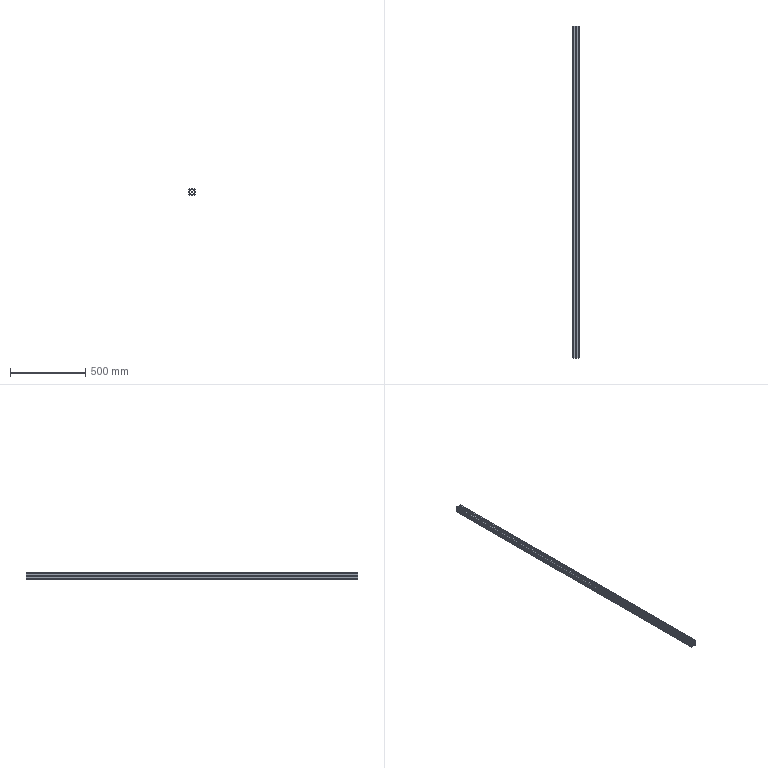Part | SolidWorks | features WeldMemberFeat 1, WeldmentFeature 1 | 1 solid | 104 faces | box 40 x 2200 x 40 mm | volume 1044704 mm3 | plane 94 | cylinder 10 | commonest cylinder face diameters 5 x4 9 x4 6.8 x2